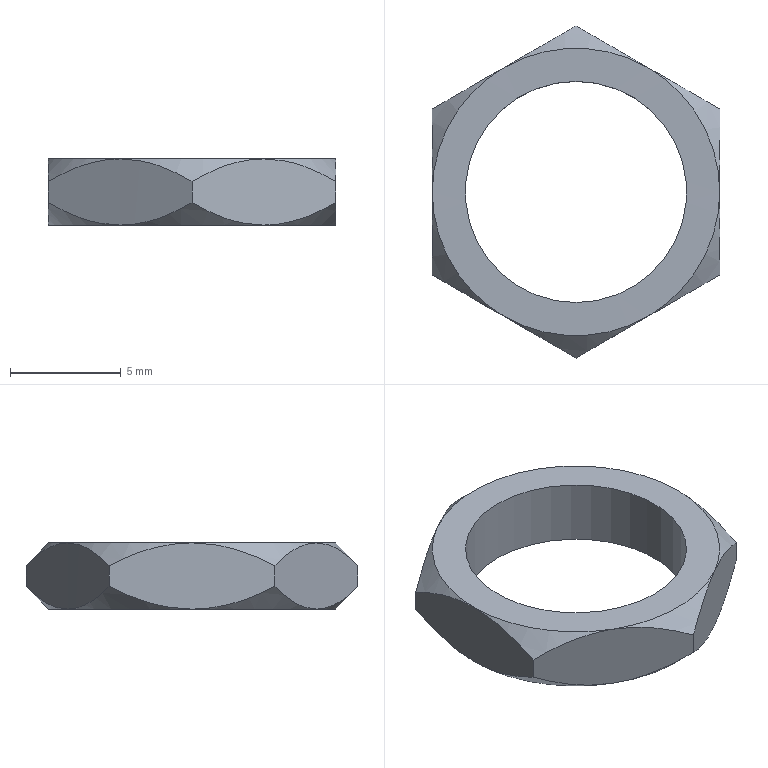Part | STEP file | 1-75.2 | 1 solid | 21 faces | box 13 x 15.011 x 3 mm | volume 194.333 mm3 | cone 12 | plane 8 | cylinder 1 | commonest cylinder face diameters 10 x1